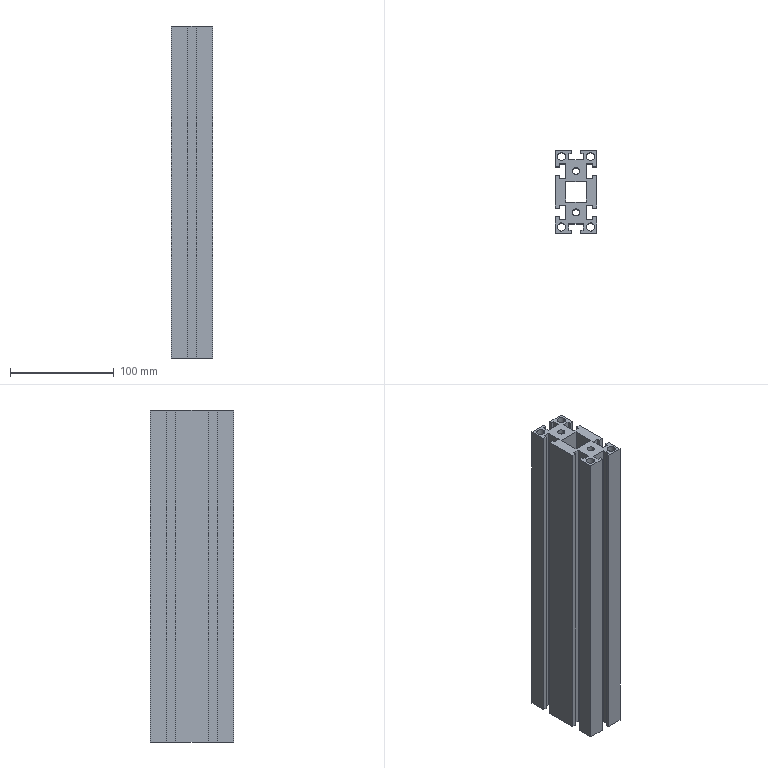Part | STEP file | PN_0074 (cross beam) | 1 solid | 86 faces | box 40 x 80 x 320 mm | volume 588947 mm3 | plane 58 | cylinder 20 | cone 8 | commonest cylinder face diameters 6.8 x8 8 x8 6.7 x4